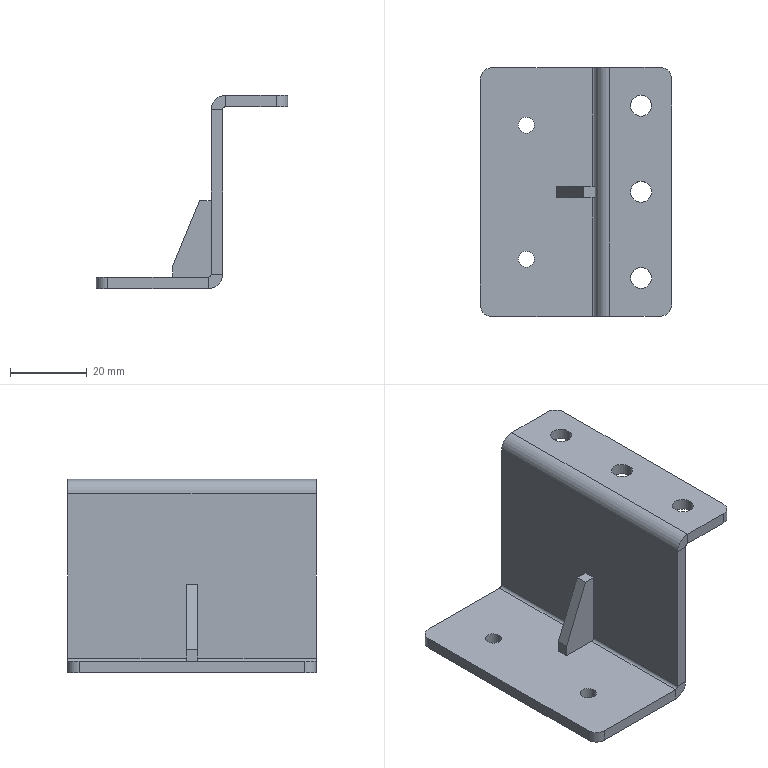Part | SolidWorks | features HoleWzd 2, Fillet 1, FlatPattern 1, ICE 1, SMBaseFlange 1, SheetMetal 1 | 1 solid | 42 faces | box 50 x 65 x 50.5 mm | volume 18737 mm3 | plane 23 | cylinder 19 | commonest cylinder face diameters 5.5 x6 4.2 x4 6 x4 1.5 x3 7.5 x2
STEP:
#1=CARTESIAN_POINT('',(-20.1,50.,-47.5));
#2=VERTEX_POINT('',#1);
#3=CARTESIAN_POINT('',(-15.9,50.,-47.5));
#4=VERTEX_POINT('',#3);
#5=CARTESIAN_POINT('',(-18.,50.,-47.5));
#6=DIRECTION('',(0.,0.,1.));
#7=DIRECTION('',(1.,0.,0.));
#8=AXIS2_PLACEMENT_3D('',#5,#6,#7);
#9=CIRCLE('',#8,2.1);
#10=EDGE_CURVE('',#2,#4,#9,.T.);
#11=ORIENTED_EDGE('',*,*,#10,.T.);
#12=CARTESIAN_POINT('',(-15.9,50.,-50.5));
#13=VERTEX_POINT('',#12);
#14=CARTESIAN_POINT('',(-15.9,50.,-50.5));
#15=DIRECTION('',(0.,0.,-1.));
#16=VECTOR('',#15,1000.);
#17=LINE('',#14,#16);
#18=EDGE_CURVE('',#4,#13,#17,.T.);
#19=ORIENTED_EDGE('',*,*,#18,.T.);
#20=CARTESIAN_POINT('',(-20.1,50.,-50.5));
#21=VERTEX_POINT('',#20);
#22=CARTESIAN_POINT('',(-18.,50.,-50.5));
#23=DIRECTION('',(0.,0.,-1.));
#24=DIRECTION('',(-1.,0.,0.));
#25=AXIS2_PLACEMENT_3D('',#22,#23,#24);
#26=CIRCLE('',#25,2.1);
#27=EDGE_CURVE('',#13,#21,#26,.T.);
#28=ORIENTED_EDGE('',*,*,#27,.T.);
#29=CARTESIAN_POINT('',(-20.1,50.,-50.5));
#30=DIRECTION('',(0.,0.,-1.));
#31=VECTOR('',#30,1000.);
#32=LINE('',#29,#31);
#33=EDGE_CURVE('',#2,#21,#32,.T.);
#34=ORIENTED_EDGE('',*,*,#33,.F.);
#35=EDGE_LOOP('',(#11,#19,#28,#34));
#36=FACE_OUTER_BOUND('',#35,.T.);
#37=CARTESIAN_POINT('',(-18.,50.,-50.5));
#38=DIRECTION('',(0.,0.,-1.));
#39=DIRECTION('',(-1.,0.,0.));
#40=AXIS2_PLACEMENT_3D('',#37,#38,#39);
#41=CYLINDRICAL_SURFACE('',#40,2.1);
#42=ADVANCED_FACE('',(#36),#41,.F.);
#43=CARTESIAN_POINT('',(-20.1,15.,-47.5));
#44=VERTEX_POINT('',#43);
#45=CARTESIAN_POINT('',(-15.9,15.,-47.5));
#46=VERTEX_POINT('',#45);
#47=CARTESIAN_POINT('',(-18.,15.,-47.5));
#48=DIRECTION('',(0.,0.,1.));
#49=DIRECTION('',(1.,0.,0.));
#50=AXIS2_PLACEMENT_3D('',#47,#48,#49);
#51=CIRCLE('',#50,2.1);
#52=EDGE_CURVE('',#44,#46,#51,.T.);
#53=ORIENTED_EDGE('',*,*,#52,.T.);
#54=CARTESIAN_POINT('',(-15.9,15.,-50.5));
#55=VERTEX_POINT('',#54);
#56=CARTESIAN_POINT('',(-15.9,15.,-50.5));
#57=DIRECTION('',(0.,0.,-1.));
#58=VECTOR('',#57,1000.);
#59=LINE('',#56,#58);
#60=EDGE_CURVE('',#46,#55,#59,.T.);
#61=ORIENTED_EDGE('',*,*,#60,.T.);
#62=CARTESIAN_POINT('',(-20.1,15.,-50.5));
#63=VERTEX_POINT('',#62);
#64=CARTESIAN_POINT('',(-18.,15.,-50.5));
#65=DIRECTION('',(0.,0.,-1.));
#66=DIRECTION('',(-1.,0.,0.));
#67=AXIS2_PLACEMENT_3D('',#64,#65,#66);
#68=CIRCLE('',#67,2.1);
#69=EDGE_CURVE('',#55,#63,#68,.T.);
#70=ORIENTED_EDGE('',*,*,#69,.T.);
#71=CARTESIAN_POINT('',(-20.1,15.,-50.5));
#72=DIRECTION('',(0.,0.,-1.));
#73=VECTOR('',#72,1000.);
#74=LINE('',#71,#73);
#75=EDGE_CURVE('',#44,#63,#74,.T.);
#76=ORIENTED_EDGE('',*,*,#75,.F.);
#77=EDGE_LOOP('',(#53,#61,#70,#76));
#78=FACE_OUTER_BOUND('',#77,.T.);
#79=CARTESIAN_POINT('',(-18.,15.,-50.5));
#80=DIRECTION('',(0.,0.,-1.));
#81=DIRECTION('',(-1.,0.,0.));
#82=AXIS2_PLACEMENT_3D('',#79,#80,#81);
#83=CYLINDRICAL_SURFACE('',#82,2.1);
#84=ADVANCED_FACE('',(#78),#83,.F.);
#85=CARTESIAN_POINT('',(9.25,55.,0.));
#86=VERTEX_POINT('',#85);
#87=CARTESIAN_POINT('',(14.75,55.,0.));
#88=VERTEX_POINT('',#87);
#89=CARTESIAN_POINT('',(12.,55.,0.));
#90=DIRECTION('',(0.,0.,1.));
#91=DIRECTION('',(1.,0.,0.));
#92=AXIS2_PLACEMENT_3D('',#89,#90,#91);
#93=CIRCLE('',#92,2.75);
#94=EDGE_CURVE('',#86,#88,#93,.T.);
#95=ORIENTED_EDGE('',*,*,#94,.T.);
#96=CARTESIAN_POINT('',(14.75,55.,-3.));
#97=VERTEX_POINT('',#96);
#98=CARTESIAN_POINT('',(14.75,55.,-3.));
#99=DIRECTION('',(0.,0.,-1.));
#100=VECTOR('',#99,1000.);
#101=LINE('',#98,#100);
#102=EDGE_CURVE('',#88,#97,#101,.T.);
#103=ORIENTED_EDGE('',*,*,#102,.T.);
#104=CARTESIAN_POINT('',(9.25,55.,-3.));
#105=VERTEX_POINT('',#104);
#106=CARTESIAN_POINT('',(12.,55.,-3.));
#107=DIRECTION('',(0.,0.,-1.));
#108=DIRECTION('',(-1.,0.,0.));
#109=AXIS2_PLACEMENT_3D('',#106,#107,#108);
#110=CIRCLE('',#109,2.75);
#111=EDGE_CURVE('',#97,#105,#110,.T.);
#112=ORIENTED_EDGE('',*,*,#111,.T.);
#113=CARTESIAN_POINT('',(9.25,55.,-3.));
#114=DIRECTION('',(0.,0.,-1.));
#115=VECTOR('',#114,1000.);
#116=LINE('',#113,#115);
#117=EDGE_CURVE('',#86,#105,#116,.T.);
#118=ORIENTED_EDGE('',*,*,#117,.F.);
#119=EDGE_LOOP('',(#95,#103,#112,#118));
#120=FACE_OUTER_BOUND('',#119,.T.);
#121=CARTESIAN_POINT('',(12.,55.,-3.));
#122=DIRECTION('',(0.,0.,-1.));
#123=DIRECTION('',(-1.,0.,0.));
#124=AXIS2_PLACEMENT_3D('',#121,#122,#123);
#125=CYLINDRICAL_SURFACE('',#124,2.75);
#126=ADVANCED_FACE('',(#120),#125,.F.);
#127=CARTESIAN_POINT('',(9.25,32.5,0.));
#128=VERTEX_POINT('',#127);
#129=CARTESIAN_POINT('',(14.75,32.5,0.));
#130=VERTEX_POINT('',#129);
#131=CARTESIAN_POINT('',(12.,32.5,0.));
#132=DIRECTION('',(0.,0.,1.));
#133=DIRECTION('',(1.,0.,0.));
#134=AXIS2_PLACEMENT_3D('',#131,#132,#133);
#135=CIRCLE('',#134,2.75);
#136=EDGE_CURVE('',#128,#130,#135,.T.);
#137=ORIENTED_EDGE('',*,*,#136,.T.);
#138=CARTESIAN_POINT('',(14.75,32.5,-3.));
#139=VERTEX_POINT('',#138);
#140=CARTESIAN_POINT('',(14.75,32.5,-3.));
#141=DIRECTION('',(0.,0.,-1.));
#142=VECTOR('',#141,1000.);
#143=LINE('',#140,#142);
#144=EDGE_CURVE('',#130,#139,#143,.T.);
#145=ORIENTED_EDGE('',*,*,#144,.T.);
#146=CARTESIAN_POINT('',(9.25,32.5,-3.));
#147=VERTEX_POINT('',#146);
#148=CARTESIAN_POINT('',(12.,32.5,-3.));
#149=DIRECTION('',(0.,0.,-1.));
#150=DIRECTION('',(-1.,0.,0.));
#151=AXIS2_PLACEMENT_3D('',#148,#149,#150);
#152=CIRCLE('',#151,2.75);
#153=EDGE_CURVE('',#139,#147,#152,.T.);
#154=ORIENTED_EDGE('',*,*,#153,.T.);
#155=CARTESIAN_POINT('',(9.25,32.5,-3.));
#156=DIRECTION('',(0.,0.,-1.));
#157=VECTOR('',#156,1000.);
#158=LINE('',#155,#157);
#159=EDGE_CURVE('',#128,#147,#158,.T.);
#160=ORIENTED_EDGE('',*,*,#159,.F.);
#161=EDGE_LOOP('',(#137,#145,#154,#160));
#162=FACE_OUTER_BOUND('',#161,.T.);
#163=CARTESIAN_POINT('',(12.,32.5,-3.));
#164=DIRECTION('',(0.,0.,-1.));
#165=DIRECTION('',(-1.,0.,0.));
#166=AXIS2_PLACEMENT_3D('',#163,#164,#165);
#167=CYLINDRICAL_SURFACE('',#166,2.75);
#168=ADVANCED_FACE('',(#162),#167,.F.);
#169=CARTESIAN_POINT('',(9.25,10.,0.));
#170=VERTEX_POINT('',#169);
#171=CARTESIAN_POINT('',(14.75,10.,0.));
#172=VERTEX_POINT('',#171);
#173=CARTESIAN_POINT('',(12.,10.,0.));
#174=DIRECTION('',(0.,0.,1.));
#175=DIRECTION('',(1.,0.,0.));
#176=AXIS2_PLACEMENT_3D('',#173,#174,#175);
#177=CIRCLE('',#176,2.75);
#178=EDGE_CURVE('',#170,#172,#177,.T.);
#179=ORIENTED_EDGE('',*,*,#178,.T.);
#180=CARTESIAN_POINT('',(14.75,10.,-3.));
#181=VERTEX_POINT('',#180);
#182=CARTESIAN_POINT('',(14.75,10.,-3.));
#183=DIRECTION('',(0.,0.,-1.));
#184=VECTOR('',#183,1000.);
#185=LINE('',#182,#184);
#186=EDGE_CURVE('',#172,#181,#185,.T.);
#187=ORIENTED_EDGE('',*,*,#186,.T.);
#188=CARTESIAN_POINT('',(9.25,10.,-3.));
#189=VERTEX_POINT('',#188);
#190=CARTESIAN_POINT('',(12.,10.,-3.));
#191=DIRECTION('',(0.,0.,-1.));
#192=DIRECTION('',(-1.,0.,0.));
#193=AXIS2_PLACEMENT_3D('',#190,#191,#192);
#194=CIRCLE('',#193,2.75);
#195=EDGE_CURVE('',#181,#189,#194,.T.);
#196=ORIENTED_EDGE('',*,*,#195,.T.);
#197=CARTESIAN_POINT('',(9.25,10.,-3.));
#198=DIRECTION('',(0.,0.,-1.));
#199=VECTOR('',#198,1000.);
#200=LINE('',#197,#199);
#201=EDGE_CURVE('',#170,#189,#200,.T.);
#202=ORIENTED_EDGE('',*,*,#201,.F.);
#203=EDGE_LOOP('',(#179,#187,#196,#202));
#204=FACE_OUTER_BOUND('',#203,.T.);
#205=CARTESIAN_POINT('',(12.,10.,-3.));
#206=DIRECTION('',(0.,0.,-1.));
#207=DIRECTION('',(-1.,0.,0.));
#208=AXIS2_PLACEMENT_3D('',#205,#206,#207);
#209=CYLINDRICAL_SURFACE('',#208,2.75);
#210=ADVANCED_FACE('',(#204),#209,.F.);
#211=CARTESIAN_POINT('',(0.,31.,-46.75));
#212=VERTEX_POINT('',#211);
#213=CARTESIAN_POINT('',(0.,0.,-46.75));
#214=VERTEX_POINT('',#213);
#215=CARTESIAN_POINT('',(0.,65.,-46.75));
#216=DIRECTION('',(0.,-1.,0.));
#217=VECTOR('',#216,1000.);
#218=LINE('',#215,#217);
#219=EDGE_CURVE('',#212,#214,#218,.T.);
#220=ORIENTED_EDGE('',*,*,#219,.F.);
#221=CARTESIAN_POINT('',(-0.75,31.,-47.5));
#222=VERTEX_POINT('',#221);
#223=CARTESIAN_POINT('',(-0.75,31.,-46.75));
#224=DIRECTION('',(0.,1.,0.));
#225=DIRECTION('',(0.,0.,1.));
#226=AXIS2_PLACEMENT_3D('',#223,#224,#225);
#227=CIRCLE('',#226,0.75);
#228=EDGE_CURVE('',#212,#222,#227,.T.);
#229=ORIENTED_EDGE('',*,*,#228,.T.);
#230=CARTESIAN_POINT('',(-0.75,0.,-47.5));
#231=VERTEX_POINT('',#230);
#232=CARTESIAN_POINT('',(-0.75,65.,-47.5));
#233=DIRECTION('',(0.,-1.,0.));
#234=VECTOR('',#233,1000.);
#235=LINE('',#232,#234);
#236=EDGE_CURVE('',#222,#231,#235,.T.);
#237=ORIENTED_EDGE('',*,*,#236,.T.);
#238=CARTESIAN_POINT('',(-0.75,0.,-46.75));
#239=DIRECTION('',(0.,1.,0.));
#240=DIRECTION('',(0.,0.,-1.));
#241=AXIS2_PLACEMENT_3D('',#238,#239,#240);
#242=CIRCLE('',#241,0.75);
#243=EDGE_CURVE('',#214,#231,#242,.T.);
#244=ORIENTED_EDGE('',*,*,#243,.F.);
#245=EDGE_LOOP('',(#220,#229,#237,#244));
#246=FACE_OUTER_BOUND('',#245,.T.);
#247=CARTESIAN_POINT('',(-0.75,65.,-46.75));
#248=DIRECTION('',(0.,-1.,0.));
#249=DIRECTION('',(0.,0.,-1.));
#250=AXIS2_PLACEMENT_3D('',#247,#248,#249);
#251=CYLINDRICAL_SURFACE('',#250,0.75);
#252=ADVANCED_FACE('',(#246),#251,.F.);
#253=CARTESIAN_POINT('',(12.,55.,-3.));
#254=DIRECTION('',(0.,0.,-1.));
#255=DIRECTION('',(-1.,0.,0.));
#256=AXIS2_PLACEMENT_3D('',#253,#254,#255);
#257=CIRCLE('',#256,2.75);
#258=EDGE_CURVE('',#105,#97,#257,.T.);
#259=ORIENTED_EDGE('',*,*,#258,.F.);
#260=ORIENTED_EDGE('',*,*,#111,.F.);
#261=EDGE_LOOP('',(#259,#260));
#262=FACE_BOUND('',#261,.T.);
#263=CARTESIAN_POINT('',(12.,32.5,-3.));
#264=DIRECTION('',(0.,0.,-1.));
#265=DIRECTION('',(-1.,0.,0.));
#266=AXIS2_PLACEMENT_3D('',#263,#264,#265);
#267=CIRCLE('',#266,2.75);
#268=EDGE_CURVE('',#147,#139,#267,.T.);
#269=ORIENTED_EDGE('',*,*,#268,.F.);
#270=ORIENTED_EDGE('',*,*,#153,.F.);
#271=EDGE_LOOP('',(#269,#270));
#272=FACE_BOUND('',#271,.T.);
#273=CARTESIAN_POINT('',(20.,62.,-3.));
#274=VERTEX_POINT('',#273);
#275=CARTESIAN_POINT('',(20.,3.,-3.));
#276=VERTEX_POINT('',#275);
#277=CARTESIAN_POINT('',(20.,65.,-3.));
#278=DIRECTION('',(0.,-1.,0.));
#279=VECTOR('',#278,1000.);
#280=LINE('',#277,#279);
#281=EDGE_CURVE('',#274,#276,#280,.T.);
#282=ORIENTED_EDGE('',*,*,#281,.T.);
#283=CARTESIAN_POINT('',(17.,0.,-3.));
#284=VERTEX_POINT('',#283);
#285=CARTESIAN_POINT('',(17.,3.,-3.));
#286=DIRECTION('',(0.,0.,-1.));
#287=DIRECTION('',(1.,0.,0.));
#288=AXIS2_PLACEMENT_3D('',#285,#286,#287);
#289=CIRCLE('',#288,3.);
#290=EDGE_CURVE('',#276,#284,#289,.T.);
#291=ORIENTED_EDGE('',*,*,#290,.T.);
#292=CARTESIAN_POINT('',(3.75,0.,-3.));
#293=VERTEX_POINT('',#292);
#294=CARTESIAN_POINT('',(20.,0.,-3.));
#295=DIRECTION('',(-1.,0.,0.));
#296=VECTOR('',#295,1000.);
#297=LINE('',#294,#296);
#298=EDGE_CURVE('',#284,#293,#297,.T.);
#299=ORIENTED_EDGE('',*,*,#298,.T.);
#300=CARTESIAN_POINT('',(3.75,65.,-3.));
#301=VERTEX_POINT('',#300);
#302=CARTESIAN_POINT('',(3.75,65.,-3.));
#303=DIRECTION('',(0.,-1.,0.));
#304=VECTOR('',#303,1000.);
#305=LINE('',#302,#304);
#306=EDGE_CURVE('',#301,#293,#305,.T.);
#307=ORIENTED_EDGE('',*,*,#306,.F.);
#308=CARTESIAN_POINT('',(17.,65.,-3.));
#309=VERTEX_POINT('',#308);
#310=CARTESIAN_POINT('',(20.,65.,-3.));
#311=DIRECTION('',(-1.,0.,0.));
#312=VECTOR('',#311,1000.);
#313=LINE('',#310,#312);
#314=EDGE_CURVE('',#309,#301,#313,.T.);
#315=ORIENTED_EDGE('',*,*,#314,.F.);
#316=CARTESIAN_POINT('',(17.,62.,-3.));
#317=DIRECTION('',(0.,0.,-1.));
#318=DIRECTION('',(1.,0.,0.));
#319=AXIS2_PLACEMENT_3D('',#316,#317,#318);
#320=CIRCLE('',#319,3.);
#321=EDGE_CURVE('',#309,#274,#320,.T.);
#322=ORIENTED_EDGE('',*,*,#321,.T.);
#323=EDGE_LOOP('',(#282,#291,#299,#307,#315,#322));
#324=FACE_OUTER_BOUND('',#323,.T.);
#325=CARTESIAN_POINT('',(12.,10.,-3.));
#326=DIRECTION('',(0.,0.,-1.));
#327=DIRECTION('',(-1.,0.,0.));
#328=AXIS2_PLACEMENT_3D('',#325,#326,#327);
#329=CIRCLE('',#328,2.75);
#330=EDGE_CURVE('',#189,#181,#329,.T.);
#331=ORIENTED_EDGE('',*,*,#330,.F.);
#332=ORIENTED_EDGE('',*,*,#195,.F.);
#333=EDGE_LOOP('',(#331,#332));
#334=FACE_BOUND('',#333,.T.);
#335=CARTESIAN_POINT('',(20.,65.,-3.));
#336=DIRECTION('',(0.,0.,1.));
#337=DIRECTION('',(1.,0.,0.));
#338=AXIS2_PLACEMENT_3D('',#335,#336,#337);
#339=PLANE('',#338);
#340=ADVANCED_FACE('',(#262,#272,#324,#334),#339,.F.);
#341=CARTESIAN_POINT('',(0.,65.,-3.75));
#342=VERTEX_POINT('',#341);
#343=CARTESIAN_POINT('',(3.,65.,-3.75));
#344=VERTEX_POINT('',#343);
#345=CARTESIAN_POINT('',(0.,65.,-3.75));
#346=DIRECTION('',(1.,0.,0.));
#347=VECTOR('',#346,1000.);
#348=LINE('',#345,#347);
#349=EDGE_CURVE('',#342,#344,#348,.T.);
#350=ORIENTED_EDGE('',*,*,#349,.F.);
#351=CARTESIAN_POINT('',(3.75,65.,0.));
#352=VERTEX_POINT('',#351);
#353=CARTESIAN_POINT('',(3.75,65.,-3.75));
#354=DIRECTION('',(0.,-1.,0.));
#355=DIRECTION('',(0.,0.,1.));
#356=AXIS2_PLACEMENT_3D('',#353,#354,#355);
#357=CIRCLE('',#356,3.75);
#358=EDGE_CURVE('',#352,#342,#357,.T.);
#359=ORIENTED_EDGE('',*,*,#358,.F.);
#360=CARTESIAN_POINT('',(3.75,65.,-3.));
#361=DIRECTION('',(0.,0.,1.));
#362=VECTOR('',#361,1000.);
#363=LINE('',#360,#362);
#364=EDGE_CURVE('',#301,#352,#363,.T.);
#365=ORIENTED_EDGE('',*,*,#364,.F.);
#366=CARTESIAN_POINT('',(3.75,65.,-3.75));
#367=DIRECTION('',(0.,-1.,0.));
#368=DIRECTION('',(1.,0.,0.));
#369=AXIS2_PLACEMENT_3D('',#366,#367,#368);
#370=CIRCLE('',#369,0.75);
#371=EDGE_CURVE('',#301,#344,#370,.T.);
#372=ORIENTED_EDGE('',*,*,#371,.T.);
#373=EDGE_LOOP('',(#350,#359,#365,#372));
#374=FACE_OUTER_BOUND('',#373,.T.);
#375=CARTESIAN_POINT('',(0.,65.,-3.75));
#376=DIRECTION('',(0.,1.,0.));
#377=DIRECTION('',(0.,0.,1.));
#378=AXIS2_PLACEMENT_3D('',#375,#376,#377);
#379=PLANE('',#378);
#380=ADVANCED_FACE('',(#374),#379,.T.);
#381=CARTESIAN_POINT('',(0.,65.,-46.75));
#382=VERTEX_POINT('',#381);
#383=CARTESIAN_POINT('',(0.,65.,0.));
#384=DIRECTION('',(0.,0.,-1.));
#385=VECTOR('',#384,1000.);
#386=LINE('',#383,#385);
#387=EDGE_CURVE('',#342,#382,#386,.T.);
#388=ORIENTED_EDGE('',*,*,#387,.F.);
#389=ORIENTED_EDGE('',*,*,#349,.T.);
#390=CARTESIAN_POINT('',(3.,65.,-46.75));
#391=VERTEX_POINT('',#390);
#392=CARTESIAN_POINT('',(3.,65.,0.));
#393=DIRECTION('',(0.,0.,-1.));
#394=VECTOR('',#393,1000.);
#395=LINE('',#392,#394);
#396=EDGE_CURVE('',#344,#391,#395,.T.);
#397=ORIENTED_EDGE('',*,*,#396,.T.);
#398=CARTESIAN_POINT('',(3.,65.,-46.75));
#399=DIRECTION('',(-1.,0.,0.));
#400=VECTOR('',#399,1000.);
#401=LINE('',#398,#400);
#402=EDGE_CURVE('',#391,#382,#401,.T.);
#403=ORIENTED_EDGE('',*,*,#402,.T.);
#404=EDGE_LOOP('',(#388,#389,#397,#403));
#405=FACE_OUTER_BOUND('',#404,.T.);
#406=CARTESIAN_POINT('',(3.75,65.,-3.));
#407=DIRECTION('',(0.,1.,0.));
#408=DIRECTION('',(0.,0.,1.));
#409=AXIS2_PLACEMENT_3D('',#406,#407,#408);
#410=PLANE('',#409);
#411=ADVANCED_FACE('',(#405),#410,.T.);
#412=CARTESIAN_POINT('',(3.75,0.,0.));
#413=VERTEX_POINT('',#412);
#414=CARTESIAN_POINT('',(3.75,0.,0.));
#415=DIRECTION('',(0.,0.,-1.));
#416=VECTOR('',#415,1000.);
#417=LINE('',#414,#416);
#418=EDGE_CURVE('',#413,#293,#417,.T.);
#419=ORIENTED_EDGE('',*,*,#418,.F.);
#420=CARTESIAN_POINT('',(0.,0.,-3.75));
#421=VERTEX_POINT('',#420);
#422=CARTESIAN_POINT('',(3.75,0.,-3.75));
#423=DIRECTION('',(0.,-1.,0.));
#424=DIRECTION('',(0.,0.,1.));
#425=AXIS2_PLACEMENT_3D('',#422,#423,#424);
#426=CIRCLE('',#425,3.75);
#427=EDGE_CURVE('',#413,#421,#426,.T.);
#428=ORIENTED_EDGE('',*,*,#427,.T.);
#429=CARTESIAN_POINT('',(3.,0.,-3.75));
#430=VERTEX_POINT('',#429);
#431=CARTESIAN_POINT('',(3.,0.,-3.75));
#432=DIRECTION('',(-1.,0.,0.));
#433=VECTOR('',#432,1000.);
#434=LINE('',#431,#433);
#435=EDGE_CURVE('',#430,#421,#434,.T.);
#436=ORIENTED_EDGE('',*,*,#435,.F.);
#437=CARTESIAN_POINT('',(3.75,0.,-3.75));
#438=DIRECTION('',(0.,-1.,0.));
#439=DIRECTION('',(1.,0.,0.));
#440=AXIS2_PLACEMENT_3D('',#437,#438,#439);
#441=CIRCLE('',#440,0.75);
#442=EDGE_CURVE('',#293,#430,#441,.T.);
#443=ORIENTED_EDGE('',*,*,#442,.F.);
#444=EDGE_LOOP('',(#419,#428,#436,#443));
#445=FACE_OUTER_BOUND('',#444,.T.);
#446=CARTESIAN_POINT('',(3.75,0.,0.));
#447=DIRECTION('',(0.,-1.,0.));
#448=DIRECTION('',(0.,0.,-1.));
#449=AXIS2_PLACEMENT_3D('',#446,#447,#448);
#450=PLANE('',#449);
#451=ADVANCED_FACE('',(#445),#450,.T.);
#452=ORIENTED_EDGE('',*,*,#298,.F.);
#453=CARTESIAN_POINT('',(17.,0.,0.));
#454=VERTEX_POINT('',#453);
#455=CARTESIAN_POINT('',(17.,0.,-3.75));
#456=DIRECTION('',(0.,0.,1.));
#457=VECTOR('',#456,1000.);
#458=LINE('',#455,#457);
#459=EDGE_CURVE('',#284,#454,#458,.T.);
#460=ORIENTED_EDGE('',*,*,#459,.T.);
#461=CARTESIAN_POINT('',(20.,0.,0.));
#462=DIRECTION('',(-1.,0.,0.));
#463=VECTOR('',#462,1000.);
#464=LINE('',#461,#463);
#465=EDGE_CURVE('',#454,#413,#464,.T.);
#466=ORIENTED_EDGE('',*,*,#465,.T.);
#467=ORIENTED_EDGE('',*,*,#418,.T.);
#468=EDGE_LOOP('',(#452,#460,#466,#467));
#469=FACE_OUTER_BOUND('',#468,.T.);
#470=CARTESIAN_POINT('',(3.,0.,-3.75));
#471=DIRECTION('',(0.,-1.,0.));
#472=DIRECTION('',(0.,0.,-1.));
#473=AXIS2_PLACEMENT_3D('',#470,#471,#472);
#474=PLANE('',#473);
#475=ADVANCED_FACE('',(#469),#474,.T.);
#476=CARTESIAN_POINT('',(-0.75,65.,-47.5));
#477=VERTEX_POINT('',#476);
#478=CARTESIAN_POINT('',(-0.75,65.,-50.5));
#479=VERTEX_POINT('',#478);
#480=CARTESIAN_POINT('',(-0.75,65.,-47.5));
#481=DIRECTION('',(0.,0.,-1.));
#482=VECTOR('',#481,1000.);
#483=LINE('',#480,#482);
#484=EDGE_CURVE('',#477,#479,#483,.T.);
#485=ORIENTED_EDGE('',*,*,#484,.F.);
#486=CARTESIAN_POINT('',(-0.75,65.,-46.75));
#487=DIRECTION('',(0.,1.,0.));
#488=DIRECTION('',(0.,0.,-1.));
#489=AXIS2_PLACEMENT_3D('',#486,#487,#488);
#490=CIRCLE('',#489,0.75);
#491=EDGE_CURVE('',#382,#477,#490,.T.);
#492=ORIENTED_EDGE('',*,*,#491,.F.);
#493=ORIENTED_EDGE('',*,*,#402,.F.);
#494=CARTESIAN_POINT('',(-0.75,65.,-46.75));
#495=DIRECTION('',(0.,1.,0.));
#496=DIRECTION('',(1.,0.,0.));
#497=AXIS2_PLACEMENT_3D('',#494,#495,#496);
#498=CIRCLE('',#497,3.75);
#499=EDGE_CURVE('',#391,#479,#498,.T.);
#500=ORIENTED_EDGE('',*,*,#499,.T.);
#501=EDGE_LOOP('',(#485,#492,#493,#500));
#502=FACE_OUTER_BOUND('',#501,.T.);
#503=CARTESIAN_POINT('',(-0.75,65.,-47.5));
#504=DIRECTION('',(0.,1.,0.));
#505=DIRECTION('',(0.,0.,1.));
#506=AXIS2_PLACEMENT_3D('',#503,#504,#505);
#507=PLANE('',#506);
#508=ADVANCED_FACE('',(#502),#507,.T.);
#509=CARTESIAN_POINT('',(-27.,65.,-50.5));
#510=VERTEX_POINT('',#509);
#511=CARTESIAN_POINT('',(0.,65.,-50.5));
#512=DIRECTION('',(-1.,0.,0.));
#513=VECTOR('',#512,1000.);
#514=LINE('',#511,#513);
#515=EDGE_CURVE('',#479,#510,#514,.T.);
#516=ORIENTED_EDGE('',*,*,#515,.T.);
#517=CARTESIAN_POINT('',(-27.,65.,-47.5));
#518=VERTEX_POINT('',#517);
#519=CARTESIAN_POINT('',(-27.,65.,-46.75));
#520=DIRECTION('',(0.,0.,1.));
#521=VECTOR('',#520,1000.);
#522=LINE('',#519,#521);
#523=EDGE_CURVE('',#510,#518,#522,.T.);
#524=ORIENTED_EDGE('',*,*,#523,.T.);
#525=CARTESIAN_POINT('',(0.,65.,-47.5));
#526=DIRECTION('',(-1.,0.,0.));
#527=VECTOR('',#526,1000.);
#528=LINE('',#525,#527);
#529=EDGE_CURVE('',#477,#518,#528,.T.);
#530=ORIENTED_EDGE('',*,*,#529,.F.);
#531=ORIENTED_EDGE('',*,*,#484,.T.);
#532=EDGE_LOOP('',(#516,#524,#530,#531));
#533=FACE_OUTER_BOUND('',#532,.T.);
#534=CARTESIAN_POINT('',(3.,65.,-46.75));
#535=DIRECTION('',(0.,1.,0.));
#536=DIRECTION('',(0.,0.,1.));
#537=AXIS2_PLACEMENT_3D('',#534,#535,#536);
#538=PLANE('',#537);
#539=ADVANCED_FACE('',(#533),#538,.T.);
#540=CARTESIAN_POINT('',(3.,0.,-46.75));
#541=VERTEX_POINT('',#540);
#542=CARTESIAN_POINT('',(0.,0.,-46.75));
#543=DIRECTION('',(1.,0.,0.));
#544=VECTOR('',#543,1000.);
#545=LINE('',#542,#544);
#546=EDGE_CURVE('',#214,#541,#545,.T.);
#547=ORIENTED_EDGE('',*,*,#546,.F.);
#548=ORIENTED_EDGE('',*,*,#243,.T.);
#549=CARTESIAN_POINT('',(-0.75,0.,-50.5));
#550=VERTEX_POINT('',#549);
#551=CARTESIAN_POINT('',(-0.75,0.,-50.5));
#552=DIRECTION('',(0.,0.,1.));
#553=VECTOR('',#552,1000.);
#554=LINE('',#551,#553);
#555=EDGE_CURVE('',#550,#231,#554,.T.);
#556=ORIENTED_EDGE('',*,*,#555,.F.);
#557=CARTESIAN_POINT('',(-0.75,0.,-46.75));
#558=DIRECTION('',(0.,1.,0.));
#559=DIRECTION('',(1.,0.,0.));
#560=AXIS2_PLACEMENT_3D('',#557,#558,#559);
#561=CIRCLE('',#560,3.75);
#562=EDGE_CURVE('',#541,#550,#561,.T.);
#563=ORIENTED_EDGE('',*,*,#562,.F.);
#564=EDGE_LOOP('',(#547,#548,#556,#563));
#565=FACE_OUTER_BOUND('',#564,.T.);
#566=CARTESIAN_POINT('',(0.,0.,-46.75));
#567=DIRECTION('',(0.,-1.,0.));
#568=DIRECTION('',(0.,0.,-1.));
#569=AXIS2_PLACEMENT_3D('',#566,#567,#568);
#570=PLANE('',#569);
#571=ADVANCED_FACE('',(#565),#570,.T.);
#572=CARTESIAN_POINT('',(0.,0.,0.));
#573=DIRECTION('',(0.,0.,-1.));
#574=VECTOR('',#573,1000.);
#575=LINE('',#572,#574);
#576=EDGE_CURVE('',#421,#214,#575,.T.);
#577=ORIENTED_EDGE('',*,*,#576,.T.);
#578=ORIENTED_EDGE('',*,*,#546,.T.);
#579=CARTESIAN_POINT('',(3.,0.,0.));
#580=DIRECTION('',(0.,0.,-1.));
#581=VECTOR('',#580,1000.);
#582=LINE('',#579,#581);
#583=EDGE_CURVE('',#430,#541,#582,.T.);
#584=ORIENTED_EDGE('',*,*,#583,.F.);
#585=ORIENTED_EDGE('',*,*,#435,.T.);
#586=EDGE_LOOP('',(#577,#578,#584,#585));
#587=FACE_OUTER_BOUND('',#586,.T.);
#588=CARTESIAN_POINT('',(-0.75,0.,-50.5));
#589=DIRECTION('',(0.,-1.,0.));
#590=DIRECTION('',(0.,0.,-1.));
#591=AXIS2_PLACEMENT_3D('',#588,#589,#590);
#592=PLANE('',#591);
#593=ADVANCED_FACE('',(#587),#592,.T.);
#594=CARTESIAN_POINT('',(-18.,50.,-50.5));
#595=DIRECTION('',(0.,0.,-1.));
#596=DIRECTION('',(-1.,0.,0.));
#597=AXIS2_PLACEMENT_3D('',#594,#595,#596);
#598=CIRCLE('',#597,2.1);
#599=EDGE_CURVE('',#21,#13,#598,.T.);
#600=ORIENTED_EDGE('',*,*,#599,.F.);
#601=ORIENTED_EDGE('',*,*,#27,.F.);
#602=EDGE_LOOP('',(#600,#601));
#603=FACE_BOUND('',#602,.T.);
#604=CARTESIAN_POINT('',(-18.,15.,-50.5));
#605=DIRECTION('',(0.,0.,-1.));
#606=DIRECTION('',(-1.,0.,0.));
#607=AXIS2_PLACEMENT_3D('',#604,#605,#606);
#608=CIRCLE('',#607,2.1);
#609=EDGE_CURVE('',#63,#55,#608,.T.);
#610=ORIENTED_EDGE('',*,*,#609,.F.);
#611=ORIENTED_EDGE('',*,*,#69,.F.);
#612=EDGE_LOOP('',(#610,#611));
#613=FACE_BOUND('',#612,.T.);
#614=CARTESIAN_POINT('',(-27.,0.,-50.5));
#615=VERTEX_POINT('',#614);
#616=CARTESIAN_POINT('',(0.,0.,-50.5));
#617=DIRECTION('',(-1.,0.,0.));
#618=VECTOR('',#617,1000.);
#619=LINE('',#616,#618);
#620=EDGE_CURVE('',#550,#615,#619,.T.);
#621=ORIENTED_EDGE('',*,*,#620,.T.);
#622=CARTESIAN_POINT('',(-30.,3.,-50.5));
#623=VERTEX_POINT('',#622);
#624=CARTESIAN_POINT('',(-27.,3.,-50.5));
#625=DIRECTION('',(0.,0.,-1.));
#626=DIRECTION('',(1.,0.,0.));
#627=AXIS2_PLACEMENT_3D('',#624,#625,#626);
#628=CIRCLE('',#627,3.);
#629=EDGE_CURVE('',#615,#623,#628,.T.);
#630=ORIENTED_EDGE('',*,*,#629,.T.);
#631=CARTESIAN_POINT('',(-30.,62.,-50.5));
#632=VERTEX_POINT('',#631);
#633=CARTESIAN_POINT('',(-30.,65.,-50.5));
#634=DIRECTION('',(0.,-1.,0.));
#635=VECTOR('',#634,1000.);
#636=LINE('',#633,#635);
#637=EDGE_CURVE('',#632,#623,#636,.T.);
#638=ORIENTED_EDGE('',*,*,#637,.F.);
#639=CARTESIAN_POINT('',(-27.,62.,-50.5));
#640=DIRECTION('',(0.,0.,-1.));
#641=DIRECTION('',(1.,0.,0.));
#642=AXIS2_PLACEMENT_3D('',#639,#640,#641);
#643=CIRCLE('',#642,3.);
#644=EDGE_CURVE('',#632,#510,#643,.T.);
#645=ORIENTED_EDGE('',*,*,#644,.T.);
#646=ORIENTED_EDGE('',*,*,#515,.F.);
#647=CARTESIAN_POINT('',(-0.75,65.,-50.5));
#648=DIRECTION('',(0.,-1.,0.));
#649=VECTOR('',#648,1000.);
#650=LINE('',#647,#649);
#651=EDGE_CURVE('',#479,#550,#650,.T.);
#652=ORIENTED_EDGE('',*,*,#651,.T.);
#653=EDGE_LOOP('',(#621,#630,#638,#645,#646,#652));
#654=FACE_OUTER_BOUND('',#653,.T.);
#655=CARTESIAN_POINT('',(0.,65.,-50.5));
#656=DIRECTION('',(0.,0.,1.));
#657=DIRECTION('',(1.,0.,0.));
#658=AXIS2_PLACEMENT_3D('',#655,#656,#657);
#659=PLANE('',#658);
#660=ADVANCED_FACE('',(#603,#613,#654),#659,.F.);
#661=ORIENTED_EDGE('',*,*,#637,.T.);
#662=CARTESIAN_POINT('',(-30.,3.,-47.5));
#663=VERTEX_POINT('',#662);
#664=CARTESIAN_POINT('',(-30.,3.,-47.5));
#665=DIRECTION('',(0.,0.,1.));
#666=VECTOR('',#665,1000.);
#667=LINE('',#664,#666);
#668=EDGE_CURVE('',#623,#663,#667,.T.);
#669=ORIENTED_EDGE('',*,*,#668,.T.);
#670=CARTESIAN_POINT('',(-30.,62.,-47.5));
#671=VERTEX_POINT('',#670);
#672=CARTESIAN_POINT('',(-30.,65.,-47.5));
#673=DIRECTION('',(0.,-1.,0.));
#674=VECTOR('',#673,1000.);
#675=LINE('',#672,#674);
#676=EDGE_CURVE('',#671,#663,#675,.T.);
#677=ORIENTED_EDGE('',*,*,#676,.F.);
#678=CARTESIAN_POINT('',(-30.,62.,-47.5));
#679=DIRECTION('',(0.,0.,-1.));
#680=VECTOR('',#679,1000.);
#681=LINE('',#678,#680);
#682=EDGE_CURVE('',#671,#632,#681,.T.);
#683=ORIENTED_EDGE('',*,*,#682,.T.);
#684=EDGE_LOOP('',(#661,#669,#677,#683));
#685=FACE_OUTER_BOUND('',#684,.T.);
#686=CARTESIAN_POINT('',(-30.,65.,-47.5));
#687=DIRECTION('',(-1.,0.,0.));
#688=DIRECTION('',(0.,0.,1.));
#689=AXIS2_PLACEMENT_3D('',#686,#687,#688);
#690=PLANE('',#689);
#691=ADVANCED_FACE('',(#685),#690,.T.);
#692=CARTESIAN_POINT('',(-0.75,34.,-47.5));
#693=VERTEX_POINT('',#692);
#694=CARTESIAN_POINT('',(-10.,34.,-47.5));
#695=VERTEX_POINT('',#694);
#696=CARTESIAN_POINT('',(-0.75,34.,-47.5));
#697=DIRECTION('',(-1.,0.,0.));
#698=VECTOR('',#697,1000.);
#699=LINE('',#696,#698);
#700=EDGE_CURVE('',#693,#695,#699,.T.);
#701=ORIENTED_EDGE('',*,*,#700,.F.);
#702=CARTESIAN_POINT('',(-0.75,65.,-47.5));
#703=DIRECTION('',(0.,-1.,0.));
#704=VECTOR('',#703,1000.);
#705=LINE('',#702,#704);
#706=EDGE_CURVE('',#477,#693,#705,.T.);
#707=ORIENTED_EDGE('',*,*,#706,.F.);
#708=ORIENTED_EDGE('',*,*,#529,.T.);
#709=CARTESIAN_POINT('',(-27.,62.,-47.5));
#710=DIRECTION('',(0.,0.,1.));
#711=DIRECTION('',(1.,0.,0.));
#712=AXIS2_PLACEMENT_3D('',#709,#710,#711);
#713=CIRCLE('',#712,3.);
#714=EDGE_CURVE('',#518,#671,#713,.T.);
#715=ORIENTED_EDGE('',*,*,#714,.T.);
#716=ORIENTED_EDGE('',*,*,#676,.T.);
#717=CARTESIAN_POINT('',(-27.,0.,-47.5));
#718=VERTEX_POINT('',#717);
#719=CARTESIAN_POINT('',(-27.,3.,-47.5));
#720=DIRECTION('',(0.,0.,1.));
#721=DIRECTION('',(1.,0.,0.));
#722=AXIS2_PLACEMENT_3D('',#719,#720,#721);
#723=CIRCLE('',#722,3.);
#724=EDGE_CURVE('',#663,#718,#723,.T.);
#725=ORIENTED_EDGE('',*,*,#724,.T.);
#726=CARTESIAN_POINT('',(0.,0.,-47.5));
#727=DIRECTION('',(-1.,0.,0.));
#728=VECTOR('',#727,1000.);
#729=LINE('',#726,#728);
#730=EDGE_CURVE('',#231,#718,#729,.T.);
#731=ORIENTED_EDGE('',*,*,#730,.F.);
#732=ORIENTED_EDGE('',*,*,#236,.F.);
#733=CARTESIAN_POINT('',(-10.,31.,-47.5));
#734=VERTEX_POINT('',#733);
#735=CARTESIAN_POINT('',(-0.75,31.,-47.5));
#736=DIRECTION('',(-1.,0.,0.));
#737=VECTOR('',#736,1000.);
#738=LINE('',#735,#737);
#739=EDGE_CURVE('',#222,#734,#738,.T.);
#740=ORIENTED_EDGE('',*,*,#739,.T.);
#741=CARTESIAN_POINT('',(-10.,34.,-47.5));
#742=DIRECTION('',(0.,-1.,0.));
#743=VECTOR('',#742,1000.);
#744=LINE('',#741,#743);
#745=EDGE_CURVE('',#695,#734,#744,.T.);
#746=ORIENTED_EDGE('',*,*,#745,.F.);
#747=EDGE_LOOP('',(#701,#707,#708,#715,#716,#725,#731,#732,#740,#746));
#748=FACE_OUTER_BOUND('',#747,.T.);
#749=ORIENTED_EDGE('',*,*,#10,.F.);
#750=CARTESIAN_POINT('',(-18.,50.,-47.5));
#751=DIRECTION('',(0.,0.,1.));
#752=DIRECTION('',(1.,0.,0.));
#753=AXIS2_PLACEMENT_3D('',#750,#751,#752);
#754=CIRCLE('',#753,2.1);
#755=EDGE_CURVE('',#4,#2,#754,.T.);
#756=ORIENTED_EDGE('',*,*,#755,.F.);
#757=EDGE_LOOP('',(#749,#756));
#758=FACE_BOUND('',#757,.T.);
#759=ORIENTED_EDGE('',*,*,#52,.F.);
#760=CARTESIAN_POINT('',(-18.,15.,-47.5));
#761=DIRECTION('',(0.,0.,1.));
#762=DIRECTION('',(1.,0.,0.));
#763=AXIS2_PLACEMENT_3D('',#760,#761,#762);
#764=CIRCLE('',#763,2.1);
#765=EDGE_CURVE('',#46,#44,#764,.T.);
#766=ORIENTED_EDGE('',*,*,#765,.F.);
#767=EDGE_LOOP('',(#759,#766));
#768=FACE_BOUND('',#767,.T.);
#769=CARTESIAN_POINT('',(0.,65.,-47.5));
#770=DIRECTION('',(0.,0.,1.));
#771=DIRECTION('',(1.,0.,0.));
#772=AXIS2_PLACEMENT_3D('',#769,#770,#771);
#773=PLANE('',#772);
#774=ADVANCED_FACE('',(#748,#758,#768),#773,.T.);
#775=CARTESIAN_POINT('',(0.,34.,-46.75));
#776=VERTEX_POINT('',#775);
#777=CARTESIAN_POINT('',(-0.75,34.,-46.75));
#778=DIRECTION('',(0.,1.,0.));
#779=DIRECTION('',(0.,0.,1.));
#780=AXIS2_PLACEMENT_3D('',#777,#778,#779);
#781=CIRCLE('',#780,0.75);
#782=EDGE_CURVE('',#776,#693,#781,.T.);
#783=ORIENTED_EDGE('',*,*,#782,.F.);
#784=CARTESIAN_POINT('',(0.,65.,-46.75));
#785=DIRECTION('',(0.,-1.,0.));
#786=VECTOR('',#785,1000.);
#787=LINE('',#784,#786);
#788=EDGE_CURVE('',#382,#776,#787,.T.);
#789=ORIENTED_EDGE('',*,*,#788,.F.);
#790=ORIENTED_EDGE('',*,*,#491,.T.);
#791=ORIENTED_EDGE('',*,*,#706,.T.);
#792=EDGE_LOOP('',(#783,#789,#790,#791));
#793=FACE_OUTER_BOUND('',#792,.T.);
#794=CARTESIAN_POINT('',(-0.75,65.,-46.75));
#795=DIRECTION('',(0.,-1.,0.));
#796=DIRECTION('',(0.,0.,-1.));
#797=AXIS2_PLACEMENT_3D('',#794,#795,#796);
#798=CYLINDRICAL_SURFACE('',#797,0.75);
#799=ADVANCED_FACE('',(#793),#798,.F.);
#800=CARTESIAN_POINT('',(0.,34.,-27.5));
#801=VERTEX_POINT('',#800);
#802=CARTESIAN_POINT('',(0.,34.,-27.5));
#803=DIRECTION('',(0.,0.,-1.));
#804=VECTOR('',#803,1000.);
#805=LINE('',#802,#804);
#806=EDGE_CURVE('',#801,#776,#805,.T.);
#807=ORIENTED_EDGE('',*,*,#806,.F.);
#808=CARTESIAN_POINT('',(0.,31.,-27.5));
#809=VERTEX_POINT('',#808);
#810=CARTESIAN_POINT('',(0.,34.,-27.5));
#811=DIRECTION('',(0.,-1.,0.));
#812=VECTOR('',#811,1000.);
#813=LINE('',#810,#812);
#814=EDGE_CURVE('',#801,#809,#813,.T.);
#815=ORIENTED_EDGE('',*,*,#814,.T.);
#816=CARTESIAN_POINT('',(0.,31.,-27.5));
#817=DIRECTION('',(0.,0.,-1.));
#818=VECTOR('',#817,1000.);
#819=LINE('',#816,#818);
#820=EDGE_CURVE('',#809,#212,#819,.T.);
#821=ORIENTED_EDGE('',*,*,#820,.T.);
#822=ORIENTED_EDGE('',*,*,#219,.T.);
#823=ORIENTED_EDGE('',*,*,#576,.F.);
#824=CARTESIAN_POINT('',(0.,65.,-3.75));
#825=DIRECTION('',(0.,-1.,0.));
#826=VECTOR('',#825,1000.);
#827=LINE('',#824,#826);
#828=EDGE_CURVE('',#342,#421,#827,.T.);
#829=ORIENTED_EDGE('',*,*,#828,.F.);
#830=ORIENTED_EDGE('',*,*,#387,.T.);
#831=ORIENTED_EDGE('',*,*,#788,.T.);
#832=EDGE_LOOP('',(#807,#815,#821,#822,#823,#829,#830,#831));
#833=FACE_OUTER_BOUND('',#832,.T.);
#834=CARTESIAN_POINT('',(0.,65.,0.));
#835=DIRECTION('',(-1.,0.,0.));
#836=DIRECTION('',(0.,0.,1.));
#837=AXIS2_PLACEMENT_3D('',#834,#835,#836);
#838=PLANE('',#837);
#839=ADVANCED_FACE('',(#833),#838,.T.);
#840=ORIENTED_EDGE('',*,*,#427,.F.);
#841=CARTESIAN_POINT('',(3.75,65.,0.));
#842=DIRECTION('',(0.,-1.,0.));
#843=VECTOR('',#842,1000.);
#844=LINE('',#841,#843);
#845=EDGE_CURVE('',#352,#413,#844,.T.);
#846=ORIENTED_EDGE('',*,*,#845,.F.);
#847=ORIENTED_EDGE('',*,*,#358,.T.);
#848=ORIENTED_EDGE('',*,*,#828,.T.);
#849=EDGE_LOOP('',(#840,#846,#847,#848));
#850=FACE_OUTER_BOUND('',#849,.T.);
#851=CARTESIAN_POINT('',(3.75,65.,-3.75));
#852=DIRECTION('',(0.,-1.,0.));
#853=DIRECTION('',(0.,0.,-1.));
#854=AXIS2_PLACEMENT_3D('',#851,#852,#853);
#855=CYLINDRICAL_SURFACE('',#854,3.75);
#856=ADVANCED_FACE('',(#850),#855,.T.);
#857=ORIENTED_EDGE('',*,*,#94,.F.);
#858=CARTESIAN_POINT('',(12.,55.,0.));
#859=DIRECTION('',(0.,0.,1.));
#860=DIRECTION('',(1.,0.,0.));
#861=AXIS2_PLACEMENT_3D('',#858,#859,#860);
#862=CIRCLE('',#861,2.75);
#863=EDGE_CURVE('',#88,#86,#862,.T.);
#864=ORIENTED_EDGE('',*,*,#863,.F.);
#865=EDGE_LOOP('',(#857,#864));
#866=FACE_BOUND('',#865,.T.);
#867=ORIENTED_EDGE('',*,*,#136,.F.);
#868=CARTESIAN_POINT('',(12.,32.5,0.));
#869=DIRECTION('',(0.,0.,1.));
#870=DIRECTION('',(1.,0.,0.));
#871=AXIS2_PLACEMENT_3D('',#868,#869,#870);
#872=CIRCLE('',#871,2.75);
#873=EDGE_CURVE('',#130,#128,#872,.T.);
#874=ORIENTED_EDGE('',*,*,#873,.F.);
#875=EDGE_LOOP('',(#867,#874));
#876=FACE_BOUND('',#875,.T.);
#877=ORIENTED_EDGE('',*,*,#178,.F.);
#878=CARTESIAN_POINT('',(12.,10.,0.));
#879=DIRECTION('',(0.,0.,1.));
#880=DIRECTION('',(1.,0.,0.));
#881=AXIS2_PLACEMENT_3D('',#878,#879,#880);
#882=CIRCLE('',#881,2.75);
#883=EDGE_CURVE('',#172,#170,#882,.T.);
#884=ORIENTED_EDGE('',*,*,#883,.F.);
#885=EDGE_LOOP('',(#877,#884));
#886=FACE_BOUND('',#885,.T.);
#887=ORIENTED_EDGE('',*,*,#465,.F.);
#888=CARTESIAN_POINT('',(20.,3.,0.));
#889=VERTEX_POINT('',#888);
#890=CARTESIAN_POINT('',(17.,3.,0.));
#891=DIRECTION('',(0.,0.,1.));
#892=DIRECTION('',(1.,0.,0.));
#893=AXIS2_PLACEMENT_3D('',#890,#891,#892);
#894=CIRCLE('',#893,3.);
#895=EDGE_CURVE('',#454,#889,#894,.T.);
#896=ORIENTED_EDGE('',*,*,#895,.T.);
#897=CARTESIAN_POINT('',(20.,62.,0.));
#898=VERTEX_POINT('',#897);
#899=CARTESIAN_POINT('',(20.,65.,0.));
#900=DIRECTION('',(0.,-1.,0.));
#901=VECTOR('',#900,1000.);
#902=LINE('',#899,#901);
#903=EDGE_CURVE('',#898,#889,#902,.T.);
#904=ORIENTED_EDGE('',*,*,#903,.F.);
#905=CARTESIAN_POINT('',(17.,65.,0.));
#906=VERTEX_POINT('',#905);
#907=CARTESIAN_POINT('',(17.,62.,0.));
#908=DIRECTION('',(0.,0.,1.));
#909=DIRECTION('',(1.,0.,0.));
#910=AXIS2_PLACEMENT_3D('',#907,#908,#909);
#911=CIRCLE('',#910,3.);
#912=EDGE_CURVE('',#898,#906,#911,.T.);
#913=ORIENTED_EDGE('',*,*,#912,.T.);
#914=CARTESIAN_POINT('',(20.,65.,0.));
#915=DIRECTION('',(-1.,0.,0.));
#916=VECTOR('',#915,1000.);
#917=LINE('',#914,#916);
#918=EDGE_CURVE('',#906,#352,#917,.T.);
#919=ORIENTED_EDGE('',*,*,#918,.T.);
#920=ORIENTED_EDGE('',*,*,#845,.T.);
#921=EDGE_LOOP('',(#887,#896,#904,#913,#919,#920));
#922=FACE_OUTER_BOUND('',#921,.T.);
#923=CARTESIAN_POINT('',(20.,65.,0.));
#924=DIRECTION('',(0.,0.,1.));
#925=DIRECTION('',(1.,0.,0.));
#926=AXIS2_PLACEMENT_3D('',#923,#924,#925);
#927=PLANE('',#926);
#928=ADVANCED_FACE('',(#866,#876,#886,#922),#927,.T.);
#929=ORIENTED_EDGE('',*,*,#903,.T.);
#930=CARTESIAN_POINT('',(20.,3.,-3.));
#931=DIRECTION('',(0.,0.,-1.));
#932=VECTOR('',#931,1000.);
#933=LINE('',#930,#932);
#934=EDGE_CURVE('',#889,#276,#933,.T.);
#935=ORIENTED_EDGE('',*,*,#934,.T.);
#936=ORIENTED_EDGE('',*,*,#281,.F.);
#937=CARTESIAN_POINT('',(20.,62.,0.));
#938=DIRECTION('',(0.,0.,1.));
#939=VECTOR('',#938,1000.);
#940=LINE('',#937,#939);
#941=EDGE_CURVE('',#274,#898,#940,.T.);
#942=ORIENTED_EDGE('',*,*,#941,.T.);
#943=EDGE_LOOP('',(#929,#935,#936,#942));
#944=FACE_OUTER_BOUND('',#943,.T.);
#945=CARTESIAN_POINT('',(20.,65.,-3.));
#946=DIRECTION('',(1.,0.,0.));
#947=DIRECTION('',(0.,0.,-1.));
#948=AXIS2_PLACEMENT_3D('',#945,#946,#947);
#949=PLANE('',#948);
#950=ADVANCED_FACE('',(#944),#949,.T.);
#951=ORIENTED_EDGE('',*,*,#442,.T.);
#952=CARTESIAN_POINT('',(3.,65.,-3.75));
#953=DIRECTION('',(0.,-1.,0.));
#954=VECTOR('',#953,1000.);
#955=LINE('',#952,#954);
#956=EDGE_CURVE('',#344,#430,#955,.T.);
#957=ORIENTED_EDGE('',*,*,#956,.F.);
#958=ORIENTED_EDGE('',*,*,#371,.F.);
#959=ORIENTED_EDGE('',*,*,#306,.T.);
#960=EDGE_LOOP('',(#951,#957,#958,#959));
#961=FACE_OUTER_BOUND('',#960,.T.);
#962=CARTESIAN_POINT('',(3.75,65.,-3.75));
#963=DIRECTION('',(0.,-1.,0.));
#964=DIRECTION('',(0.,0.,-1.));
#965=AXIS2_PLACEMENT_3D('',#962,#963,#964);
#966=CYLINDRICAL_SURFACE('',#965,0.75);
#967=ADVANCED_FACE('',(#961),#966,.F.);
#968=ORIENTED_EDGE('',*,*,#583,.T.);
#969=CARTESIAN_POINT('',(3.,65.,-46.75));
#970=DIRECTION('',(0.,-1.,0.));
#971=VECTOR('',#970,1000.);
#972=LINE('',#969,#971);
#973=EDGE_CURVE('',#391,#541,#972,.T.);
#974=ORIENTED_EDGE('',*,*,#973,.F.);
#975=ORIENTED_EDGE('',*,*,#396,.F.);
#976=ORIENTED_EDGE('',*,*,#956,.T.);
#977=EDGE_LOOP('',(#968,#974,#975,#976));
#978=FACE_OUTER_BOUND('',#977,.T.);
#979=CARTESIAN_POINT('',(3.,65.,0.));
#980=DIRECTION('',(-1.,0.,0.));
#981=DIRECTION('',(0.,0.,1.));
#982=AXIS2_PLACEMENT_3D('',#979,#980,#981);
#983=PLANE('',#982);
#984=ADVANCED_FACE('',(#978),#983,.F.);
#985=ORIENTED_EDGE('',*,*,#562,.T.);
#986=ORIENTED_EDGE('',*,*,#651,.F.);
#987=ORIENTED_EDGE('',*,*,#499,.F.);
#988=ORIENTED_EDGE('',*,*,#973,.T.);
#989=EDGE_LOOP('',(#985,#986,#987,#988));
#990=FACE_OUTER_BOUND('',#989,.T.);
#991=CARTESIAN_POINT('',(-0.75,65.,-46.75));
#992=DIRECTION('',(0.,-1.,0.));
#993=DIRECTION('',(0.,0.,-1.));
#994=AXIS2_PLACEMENT_3D('',#991,#992,#993);
#995=CYLINDRICAL_SURFACE('',#994,3.75);
#996=ADVANCED_FACE('',(#990),#995,.T.);
#997=ORIENTED_EDGE('',*,*,#918,.F.);
#998=CARTESIAN_POINT('',(17.,65.,-3.));
#999=DIRECTION('',(0.,0.,-1.));
#1000=VECTOR('',#999,1000.);
#1001=LINE('',#998,#1000);
#1002=EDGE_CURVE('',#906,#309,#1001,.T.);
#1003=ORIENTED_EDGE('',*,*,#1002,.T.);
#1004=ORIENTED_EDGE('',*,*,#314,.T.);
#1005=ORIENTED_EDGE('',*,*,#364,.T.);
#1006=EDGE_LOOP('',(#997,#1003,#1004,#1005));
#1007=FACE_OUTER_BOUND('',#1006,.T.);
#1008=CARTESIAN_POINT('',(-0.75,65.,-46.75));
#1009=DIRECTION('',(0.,-1.,0.));
#1010=DIRECTION('',(-1.,0.,0.));
#1011=AXIS2_PLACEMENT_3D('',#1008,#1009,#1010);
#1012=PLANE('',#1011);
#1013=ADVANCED_FACE('',(#1007),#1012,.F.);
#1014=ORIENTED_EDGE('',*,*,#730,.T.);
#1015=CARTESIAN_POINT('',(-27.,0.,-46.75));
#1016=DIRECTION('',(0.,0.,-1.));
#1017=VECTOR('',#1016,1000.);
#1018=LINE('',#1015,#1017);
#1019=EDGE_CURVE('',#718,#615,#1018,.T.);
#1020=ORIENTED_EDGE('',*,*,#1019,.T.);
#1021=ORIENTED_EDGE('',*,*,#620,.F.);
#1022=ORIENTED_EDGE('',*,*,#555,.T.);
#1023=EDGE_LOOP('',(#1014,#1020,#1021,#1022));
#1024=FACE_OUTER_BOUND('',#1023,.T.);
#1025=CARTESIAN_POINT('',(-0.75,0.,-46.75));
#1026=DIRECTION('',(0.,-1.,0.));
#1027=DIRECTION('',(-1.,0.,0.));
#1028=AXIS2_PLACEMENT_3D('',#1025,#1026,#1027);
#1029=PLANE('',#1028);
#1030=ADVANCED_FACE('',(#1024),#1029,.T.);
#1031=ORIENTED_EDGE('',*,*,#724,.F.);
#1032=ORIENTED_EDGE('',*,*,#668,.F.);
#1033=ORIENTED_EDGE('',*,*,#629,.F.);
#1034=ORIENTED_EDGE('',*,*,#1019,.F.);
#1035=EDGE_LOOP('',(#1031,#1032,#1033,#1034));
#1036=FACE_OUTER_BOUND('',#1035,.T.);
#1037=CARTESIAN_POINT('',(-27.,3.,-46.75));
#1038=DIRECTION('',(0.,0.,-1.));
#1039=DIRECTION('',(-1.,0.,0.));
#1040=AXIS2_PLACEMENT_3D('',#1037,#1038,#1039);
#1041=CYLINDRICAL_SURFACE('',#1040,3.);
#1042=ADVANCED_FACE('',(#1036),#1041,.T.);
#1043=ORIENTED_EDGE('',*,*,#714,.F.);
#1044=ORIENTED_EDGE('',*,*,#523,.F.);
#1045=ORIENTED_EDGE('',*,*,#644,.F.);
#1046=ORIENTED_EDGE('',*,*,#682,.F.);
#1047=EDGE_LOOP('',(#1043,#1044,#1045,#1046));
#1048=FACE_OUTER_BOUND('',#1047,.T.);
#1049=CARTESIAN_POINT('',(-27.,62.,-47.5));
#1050=DIRECTION('',(0.,0.,-1.));
#1051=DIRECTION('',(-1.,0.,0.));
#1052=AXIS2_PLACEMENT_3D('',#1049,#1050,#1051);
#1053=CYLINDRICAL_SURFACE('',#1052,3.);
#1054=ADVANCED_FACE('',(#1048),#1053,.T.);
#1055=ORIENTED_EDGE('',*,*,#290,.F.);
#1056=ORIENTED_EDGE('',*,*,#934,.F.);
#1057=ORIENTED_EDGE('',*,*,#895,.F.);
#1058=ORIENTED_EDGE('',*,*,#459,.F.);
#1059=EDGE_LOOP('',(#1055,#1056,#1057,#1058));
#1060=FACE_OUTER_BOUND('',#1059,.T.);
#1061=CARTESIAN_POINT('',(17.,3.,-3.75));
#1062=DIRECTION('',(0.,0.,1.));
#1063=DIRECTION('',(1.,0.,0.));
#1064=AXIS2_PLACEMENT_3D('',#1061,#1062,#1063);
#1065=CYLINDRICAL_SURFACE('',#1064,3.);
#1066=ADVANCED_FACE('',(#1060),#1065,.T.);
#1067=ORIENTED_EDGE('',*,*,#321,.F.);
#1068=ORIENTED_EDGE('',*,*,#1002,.F.);
#1069=ORIENTED_EDGE('',*,*,#912,.F.);
#1070=ORIENTED_EDGE('',*,*,#941,.F.);
#1071=EDGE_LOOP('',(#1067,#1068,#1069,#1070));
#1072=FACE_OUTER_BOUND('',#1071,.T.);
#1073=CARTESIAN_POINT('',(17.,62.,-3.));
#1074=DIRECTION('',(0.,0.,-1.));
#1075=DIRECTION('',(-1.,0.,0.));
#1076=AXIS2_PLACEMENT_3D('',#1073,#1074,#1075);
#1077=CYLINDRICAL_SURFACE('',#1076,3.);
#1078=ADVANCED_FACE('',(#1072),#1077,.T.);
#1079=ORIENTED_EDGE('',*,*,#186,.F.);
#1080=ORIENTED_EDGE('',*,*,#883,.T.);
#1081=ORIENTED_EDGE('',*,*,#201,.T.);
#1082=ORIENTED_EDGE('',*,*,#330,.T.);
#1083=EDGE_LOOP('',(#1079,#1080,#1081,#1082));
#1084=FACE_OUTER_BOUND('',#1083,.T.);
#1085=CARTESIAN_POINT('',(12.,10.,-3.));
#1086=DIRECTION('',(0.,0.,-1.));
#1087=DIRECTION('',(-1.,0.,0.));
#1088=AXIS2_PLACEMENT_3D('',#1085,#1086,#1087);
#1089=CYLINDRICAL_SURFACE('',#1088,2.75);
#1090=ADVANCED_FACE('',(#1084),#1089,.F.);
#1091=ORIENTED_EDGE('',*,*,#144,.F.);
#1092=ORIENTED_EDGE('',*,*,#873,.T.);
#1093=ORIENTED_EDGE('',*,*,#159,.T.);
#1094=ORIENTED_EDGE('',*,*,#268,.T.);
#1095=EDGE_LOOP('',(#1091,#1092,#1093,#1094));
#1096=FACE_OUTER_BOUND('',#1095,.T.);
#1097=CARTESIAN_POINT('',(12.,32.5,-3.));
#1098=DIRECTION('',(0.,0.,-1.));
#1099=DIRECTION('',(-1.,0.,0.));
#1100=AXIS2_PLACEMENT_3D('',#1097,#1098,#1099);
#1101=CYLINDRICAL_SURFACE('',#1100,2.75);
#1102=ADVANCED_FACE('',(#1096),#1101,.F.);
#1103=ORIENTED_EDGE('',*,*,#102,.F.);
#1104=ORIENTED_EDGE('',*,*,#863,.T.);
#1105=ORIENTED_EDGE('',*,*,#117,.T.);
#1106=ORIENTED_EDGE('',*,*,#258,.T.);
#1107=EDGE_LOOP('',(#1103,#1104,#1105,#1106));
#1108=FACE_OUTER_BOUND('',#1107,.T.);
#1109=CARTESIAN_POINT('',(12.,55.,-3.));
#1110=DIRECTION('',(0.,0.,-1.));
#1111=DIRECTION('',(-1.,0.,0.));
#1112=AXIS2_PLACEMENT_3D('',#1109,#1110,#1111);
#1113=CYLINDRICAL_SURFACE('',#1112,2.75);
#1114=ADVANCED_FACE('',(#1108),#1113,.F.);
#1115=ORIENTED_EDGE('',*,*,#60,.F.);
#1116=ORIENTED_EDGE('',*,*,#765,.T.);
#1117=ORIENTED_EDGE('',*,*,#75,.T.);
#1118=ORIENTED_EDGE('',*,*,#609,.T.);
#1119=EDGE_LOOP('',(#1115,#1116,#1117,#1118));
#1120=FACE_OUTER_BOUND('',#1119,.T.);
#1121=CARTESIAN_POINT('',(-18.,15.,-50.5));
#1122=DIRECTION('',(0.,0.,-1.));
#1123=DIRECTION('',(-1.,0.,0.));
#1124=AXIS2_PLACEMENT_3D('',#1121,#1122,#1123);
#1125=CYLINDRICAL_SURFACE('',#1124,2.1);
#1126=ADVANCED_FACE('',(#1120),#1125,.F.);
#1127=ORIENTED_EDGE('',*,*,#18,.F.);
#1128=ORIENTED_EDGE('',*,*,#755,.T.);
#1129=ORIENTED_EDGE('',*,*,#33,.T.);
#1130=ORIENTED_EDGE('',*,*,#599,.T.);
#1131=EDGE_LOOP('',(#1127,#1128,#1129,#1130));
#1132=FACE_OUTER_BOUND('',#1131,.T.);
#1133=CARTESIAN_POINT('',(-18.,50.,-50.5));
#1134=DIRECTION('',(0.,0.,-1.));
#1135=DIRECTION('',(-1.,0.,0.));
#1136=AXIS2_PLACEMENT_3D('',#1133,#1134,#1135);
#1137=CYLINDRICAL_SURFACE('',#1136,2.1);
#1138=ADVANCED_FACE('',(#1132),#1137,.F.);
#1139=CARTESIAN_POINT('',(-10.,31.,-44.5));
#1140=VERTEX_POINT('',#1139);
#1141=CARTESIAN_POINT('',(-10.,31.,-47.5));
#1142=DIRECTION('',(0.,0.,1.));
#1143=VECTOR('',#1142,1000.);
#1144=LINE('',#1141,#1143);
#1145=EDGE_CURVE('',#734,#1140,#1144,.T.);
#1146=ORIENTED_EDGE('',*,*,#1145,.T.);
#1147=CARTESIAN_POINT('',(-10.,34.,-44.5));
#1148=VERTEX_POINT('',#1147);
#1149=CARTESIAN_POINT('',(-10.,34.,-44.5));
#1150=DIRECTION('',(0.,-1.,0.));
#1151=VECTOR('',#1150,1000.);
#1152=LINE('',#1149,#1151);
#1153=EDGE_CURVE('',#1148,#1140,#1152,.T.);
#1154=ORIENTED_EDGE('',*,*,#1153,.F.);
#1155=CARTESIAN_POINT('',(-10.,34.,-47.5));
#1156=DIRECTION('',(0.,0.,1.));
#1157=VECTOR('',#1156,1000.);
#1158=LINE('',#1155,#1157);
#1159=EDGE_CURVE('',#695,#1148,#1158,.T.);
#1160=ORIENTED_EDGE('',*,*,#1159,.F.);
#1161=ORIENTED_EDGE('',*,*,#745,.T.);
#1162=EDGE_LOOP('',(#1146,#1154,#1160,#1161));
#1163=FACE_OUTER_BOUND('',#1162,.T.);
#1164=CARTESIAN_POINT('',(-10.,34.,-47.5));
#1165=DIRECTION('',(1.,0.,0.));
#1166=DIRECTION('',(0.,0.,-1.));
#1167=AXIS2_PLACEMENT_3D('',#1164,#1165,#1166);
#1168=PLANE('',#1167);
#1169=ADVANCED_FACE('',(#1163),#1168,.F.);
#1170=CARTESIAN_POINT('',(-3.,31.,-27.5));
#1171=VERTEX_POINT('',#1170);
#1172=CARTESIAN_POINT('',(-10.,31.,-44.5));
#1173=DIRECTION('',(0.3807,0.,0.9247));
#1174=VECTOR('',#1173,1000.);
#1175=LINE('',#1172,#1174);
#1176=EDGE_CURVE('',#1140,#1171,#1175,.T.);
#1177=ORIENTED_EDGE('',*,*,#1176,.T.);
#1178=CARTESIAN_POINT('',(-3.,34.,-27.5));
#1179=VERTEX_POINT('',#1178);
#1180=CARTESIAN_POINT('',(-3.,34.,-27.5));
#1181=DIRECTION('',(0.,-1.,0.));
#1182=VECTOR('',#1181,1000.);
#1183=LINE('',#1180,#1182);
#1184=EDGE_CURVE('',#1179,#1171,#1183,.T.);
#1185=ORIENTED_EDGE('',*,*,#1184,.F.);
#1186=CARTESIAN_POINT('',(-10.,34.,-44.5));
#1187=DIRECTION('',(0.3807,0.,0.9247));
#1188=VECTOR('',#1187,1000.);
#1189=LINE('',#1186,#1188);
#1190=EDGE_CURVE('',#1148,#1179,#1189,.T.);
#1191=ORIENTED_EDGE('',*,*,#1190,.F.);
#1192=ORIENTED_EDGE('',*,*,#1153,.T.);
#1193=EDGE_LOOP('',(#1177,#1185,#1191,#1192));
#1194=FACE_OUTER_BOUND('',#1193,.T.);
#1195=CARTESIAN_POINT('',(-10.,34.,-44.5));
#1196=DIRECTION('',(0.9247,0.,-0.3807));
#1197=DIRECTION('',(-0.3807,0.,-0.9247));
#1198=AXIS2_PLACEMENT_3D('',#1195,#1196,#1197);
#1199=PLANE('',#1198);
#1200=ADVANCED_FACE('',(#1194),#1199,.F.);
#1201=CARTESIAN_POINT('',(-3.,31.,-27.5));
#1202=DIRECTION('',(1.,0.,0.));
#1203=VECTOR('',#1202,1000.);
#1204=LINE('',#1201,#1203);
#1205=EDGE_CURVE('',#1171,#809,#1204,.T.);
#1206=ORIENTED_EDGE('',*,*,#1205,.T.);
#1207=ORIENTED_EDGE('',*,*,#814,.F.);
#1208=CARTESIAN_POINT('',(-3.,34.,-27.5));
#1209=DIRECTION('',(1.,0.,0.));
#1210=VECTOR('',#1209,1000.);
#1211=LINE('',#1208,#1210);
#1212=EDGE_CURVE('',#1179,#801,#1211,.T.);
#1213=ORIENTED_EDGE('',*,*,#1212,.F.);
#1214=ORIENTED_EDGE('',*,*,#1184,.T.);
#1215=EDGE_LOOP('',(#1206,#1207,#1213,#1214));
#1216=FACE_OUTER_BOUND('',#1215,.T.);
#1217=CARTESIAN_POINT('',(-3.,34.,-27.5));
#1218=DIRECTION('',(0.,0.,-1.));
#1219=DIRECTION('',(-1.,0.,0.));
#1220=AXIS2_PLACEMENT_3D('',#1217,#1218,#1219);
#1221=PLANE('',#1220);
#1222=ADVANCED_FACE('',(#1216),#1221,.F.);
#1223=ORIENTED_EDGE('',*,*,#1159,.T.);
#1224=ORIENTED_EDGE('',*,*,#1190,.T.);
#1225=ORIENTED_EDGE('',*,*,#1212,.T.);
#1226=ORIENTED_EDGE('',*,*,#806,.T.);
#1227=ORIENTED_EDGE('',*,*,#782,.T.);
#1228=ORIENTED_EDGE('',*,*,#700,.T.);
#1229=EDGE_LOOP('',(#1223,#1224,#1225,#1226,#1227,#1228));
#1230=FACE_OUTER_BOUND('',#1229,.T.);
#1231=CARTESIAN_POINT('',(-0.75,34.,-46.75));
#1232=DIRECTION('',(0.,1.,0.));
#1233=DIRECTION('',(0.,0.,1.));
#1234=AXIS2_PLACEMENT_3D('',#1231,#1232,#1233);
#1235=PLANE('',#1234);
#1236=ADVANCED_FACE('',(#1230),#1235,.T.);
#1237=ORIENTED_EDGE('',*,*,#1145,.F.);
#1238=ORIENTED_EDGE('',*,*,#739,.F.);
#1239=ORIENTED_EDGE('',*,*,#228,.F.);
#1240=ORIENTED_EDGE('',*,*,#820,.F.);
#1241=ORIENTED_EDGE('',*,*,#1205,.F.);
#1242=ORIENTED_EDGE('',*,*,#1176,.F.);
#1243=EDGE_LOOP('',(#1237,#1238,#1239,#1240,#1241,#1242));
#1244=FACE_OUTER_BOUND('',#1243,.T.);
#1245=CARTESIAN_POINT('',(-0.75,31.,-46.75));
#1246=DIRECTION('',(0.,1.,0.));
#1247=DIRECTION('',(0.,0.,1.));
#1248=AXIS2_PLACEMENT_3D('',#1245,#1246,#1247);
#1249=PLANE('',#1248);
#1250=ADVANCED_FACE('',(#1244),#1249,.F.);
#1251=CLOSED_SHELL('',(#42,#84,#126,#168,#210,#252,#340,#380,#411,#451,#475,#508,#539,#571,#593,#660,#691,#774,#799,#839,#856,#928,#950,#967,#984,#996,#1013,#1030,#1042,#1054,#1066,#1078,#1090,#1102,#1114,#1126,#1138,#1169,#1200,#1222,#1236,#1250));
#1252=MANIFOLD_SOLID_BREP('',#1251);
#1253=CARTESIAN_POINT('',(0.,0.,0.));
#1254=DIRECTION('',(0.,0.,1.));
#1255=DIRECTION('',(1.,0.,0.));
#1256=AXIS2_PLACEMENT_3D('',#1253,#1254,#1255);
#1257=(LENGTH_UNIT()NAMED_UNIT(*)SI_UNIT(.MILLI.,.METRE.));
#1258=UNCERTAINTY_MEASURE_WITH_UNIT(LENGTH_MEASURE(0.00001),#1257,'','');
#1259=(NAMED_UNIT(*)PLANE_ANGLE_UNIT()SI_UNIT($,.RADIAN.));
#1260=(NAMED_UNIT(*)SI_UNIT($,.STERADIAN.)SOLID_ANGLE_UNIT());
#1261=(GEOMETRIC_REPRESENTATION_CONTEXT(3)GLOBAL_UNCERTAINTY_ASSIGNED_CONTEXT((#1258))GLOBAL_UNIT_ASSIGNED_CONTEXT((#1257,#1259,#1260))REPRESENTATION_CONTEXT('',''));
#1262=ADVANCED_BREP_SHAPE_REPRESENTATION('',(#1252,#1256),#1261);